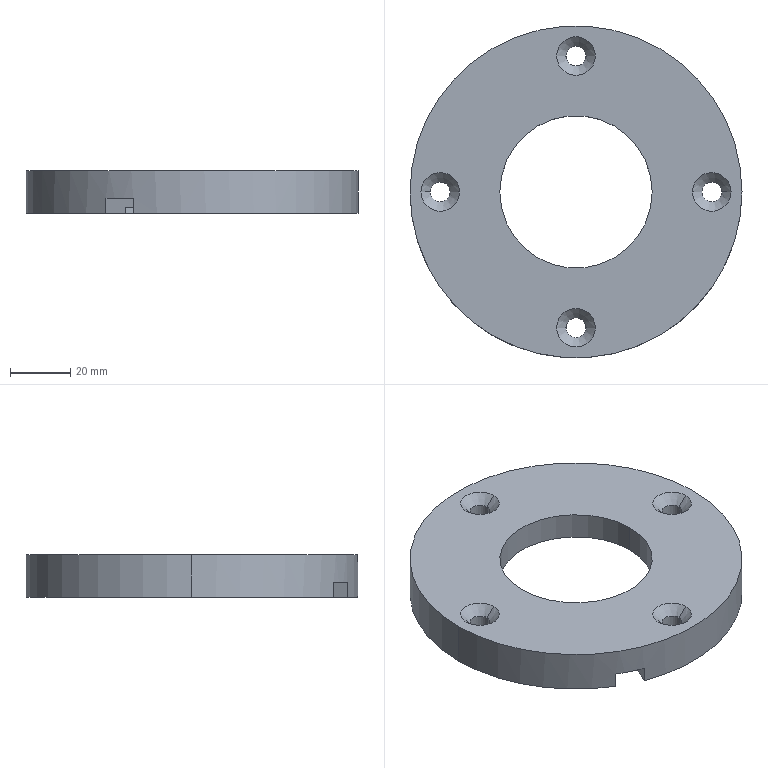Part | STEP file | Gland cover SGN-4-04 | 1 solid | 32 faces | box 110 x 110 x 14 mm | volume 91595 mm3 | cylinder 18 | cone 8 | plane 6 | commonest cylinder face diameters 6.6 x8 65 x3 80 x3 50.5 x2 110 x2